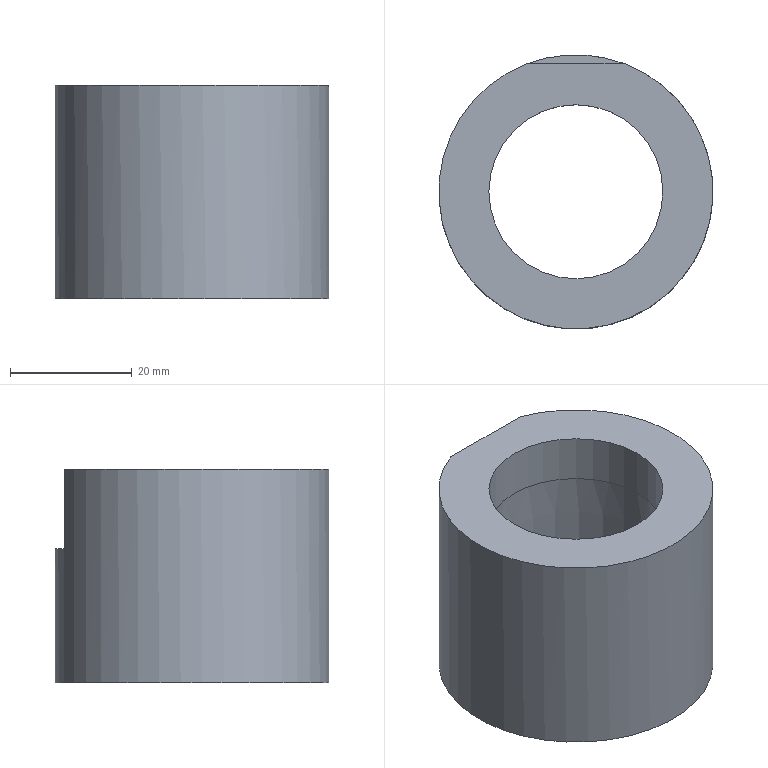Part | STEP file | lll_id4046_x_t | 1 solid | 7 faces | box 45 x 45 x 35 mm | volume 32145 mm3 | plane 4 | cylinder 2 | cone 1 | commonest cylinder face diameters 28.57 x1 45 x1
STEP:
#1=CARTESIAN_POINT('',(3205.477,-41.296,-35.));
#2=VERTEX_POINT('',#1);
#3=CARTESIAN_POINT('',(3205.477,-56.288,-35.));
#4=DIRECTION('',(0.,0.,-1.));
#5=DIRECTION('',(0.,1.,0.));
#6=AXIS2_PLACEMENT_3D('',#3,#4,#5);
#7=CIRCLE('',#6,14.992);
#8=EDGE_CURVE('',#2,#2,#7,.T.);
#9=ORIENTED_EDGE('',*,*,#8,.F.);
#10=EDGE_LOOP('',(#9));
#11=FACE_BOUND('',#10,.T.);
#12=CARTESIAN_POINT('',(3205.477,-33.788,-35.));
#13=VERTEX_POINT('',#12);
#14=CARTESIAN_POINT('',(3205.477,-56.288,-35.));
#15=DIRECTION('',(0.,0.,-1.));
#16=DIRECTION('',(0.,1.,0.));
#17=AXIS2_PLACEMENT_3D('',#14,#15,#16);
#18=CIRCLE('',#17,22.5);
#19=EDGE_CURVE('',#13,#13,#18,.T.);
#20=ORIENTED_EDGE('',*,*,#19,.T.);
#21=EDGE_LOOP('',(#20));
#22=FACE_BOUND('',#21,.T.);
#23=CARTESIAN_POINT('',(3199.977,-56.288,-35.));
#24=DIRECTION('',(0.,0.,-1.));
#25=DIRECTION('',(1.,0.,0.));
#26=AXIS2_PLACEMENT_3D('',#23,#24,#25);
#27=PLANE('',#26);
#28=ADVANCED_FACE('',(#11,#22),#27,.T.);
#29=CARTESIAN_POINT('',(3205.477,-42.003,-8.));
#30=VERTEX_POINT('',#29);
#31=CARTESIAN_POINT('',(3205.477,-56.288,-8.));
#32=DIRECTION('',(0.,0.,1.));
#33=DIRECTION('',(0.,1.,0.));
#34=AXIS2_PLACEMENT_3D('',#31,#32,#33);
#35=CIRCLE('',#34,14.285);
#36=EDGE_CURVE('',#30,#30,#35,.T.);
#37=ORIENTED_EDGE('',*,*,#36,.F.);
#38=EDGE_LOOP('',(#37));
#39=FACE_BOUND('',#38,.T.);
#40=CARTESIAN_POINT('',(3205.477,-42.003,0.00001711));
#41=VERTEX_POINT('',#40);
#42=CARTESIAN_POINT('',(3205.477,-56.288,0.00001711));
#43=DIRECTION('',(0.,0.,-1.));
#44=DIRECTION('',(0.,1.,0.));
#45=AXIS2_PLACEMENT_3D('',#42,#43,#44);
#46=CIRCLE('',#45,14.285);
#47=EDGE_CURVE('',#41,#41,#46,.T.);
#48=ORIENTED_EDGE('',*,*,#47,.F.);
#49=EDGE_LOOP('',(#48));
#50=FACE_BOUND('',#49,.T.);
#51=CARTESIAN_POINT('',(3205.477,-56.288,-2.4));
#52=DIRECTION('',(0.,0.,1.));
#53=DIRECTION('',(0.,1.,0.));
#54=AXIS2_PLACEMENT_3D('',#51,#52,#53);
#55=CYLINDRICAL_SURFACE('',#54,14.285);
#56=ADVANCED_FACE('',(#39,#50),#55,.F.);
#57=CARTESIAN_POINT('',(3213.554,-35.288,0.00001711));
#58=VERTEX_POINT('',#57);
#59=CARTESIAN_POINT('',(3197.399,-35.288,0.00001711));
#60=VERTEX_POINT('',#59);
#61=CARTESIAN_POINT('',(3205.477,-35.288,0.00001711));
#62=DIRECTION('',(-1.,0.,0.));
#63=VECTOR('',#62,1.);
#64=LINE('',#61,#63);
#65=EDGE_CURVE('',#58,#60,#64,.T.);
#66=ORIENTED_EDGE('',*,*,#65,.T.);
#67=CARTESIAN_POINT('',(3205.477,-56.288,0.00001711));
#68=DIRECTION('',(0.,0.,-1.));
#69=DIRECTION('',(0.,1.,0.));
#70=AXIS2_PLACEMENT_3D('',#67,#68,#69);
#71=CIRCLE('',#70,22.5);
#72=EDGE_CURVE('',#58,#60,#71,.T.);
#73=ORIENTED_EDGE('',*,*,#72,.F.);
#74=EDGE_LOOP('',(#66,#73));
#75=FACE_BOUND('',#74,.T.);
#76=ORIENTED_EDGE('',*,*,#47,.T.);
#77=EDGE_LOOP('',(#76));
#78=FACE_BOUND('',#77,.T.);
#79=CARTESIAN_POINT('',(3205.477,-56.288,0.00001711));
#80=DIRECTION('',(0.,0.,1.));
#81=DIRECTION('',(0.,-1.,0.));
#82=AXIS2_PLACEMENT_3D('',#79,#80,#81);
#83=PLANE('',#82);
#84=ADVANCED_FACE('',(#75,#78),#83,.T.);
#85=ORIENTED_EDGE('',*,*,#19,.F.);
#86=EDGE_LOOP('',(#85));
#87=FACE_BOUND('',#86,.T.);
#88=ORIENTED_EDGE('',*,*,#72,.T.);
#89=CARTESIAN_POINT('',(3197.399,-35.288,-13.));
#90=VERTEX_POINT('',#89);
#91=CARTESIAN_POINT('',(3197.399,-35.288,-15.));
#92=DIRECTION('',(0.,0.,-1.));
#93=VECTOR('',#92,1.);
#94=LINE('',#91,#93);
#95=EDGE_CURVE('',#60,#90,#94,.T.);
#96=ORIENTED_EDGE('',*,*,#95,.T.);
#97=CARTESIAN_POINT('',(3213.554,-35.288,-13.));
#98=VERTEX_POINT('',#97);
#99=CARTESIAN_POINT('',(3205.477,-56.288,-13.));
#100=DIRECTION('',(0.,0.,-1.));
#101=DIRECTION('',(0.,-1.,0.));
#102=AXIS2_PLACEMENT_3D('',#99,#100,#101);
#103=CIRCLE('',#102,22.5);
#104=EDGE_CURVE('',#90,#98,#103,.T.);
#105=ORIENTED_EDGE('',*,*,#104,.T.);
#106=CARTESIAN_POINT('',(3213.554,-35.288,-15.));
#107=DIRECTION('',(0.,0.,1.));
#108=VECTOR('',#107,1.);
#109=LINE('',#106,#108);
#110=EDGE_CURVE('',#98,#58,#109,.T.);
#111=ORIENTED_EDGE('',*,*,#110,.T.);
#112=EDGE_LOOP('',(#88,#96,#105,#111));
#113=FACE_BOUND('',#112,.T.);
#114=CARTESIAN_POINT('',(3205.477,-56.288,-15.));
#115=DIRECTION('',(0.,0.,-1.));
#116=DIRECTION('',(-1.,0.,0.));
#117=AXIS2_PLACEMENT_3D('',#114,#115,#116);
#118=CYLINDRICAL_SURFACE('',#117,22.5);
#119=ADVANCED_FACE('',(#87,#113),#118,.T.);
#120=CARTESIAN_POINT('',(3205.477,-35.288,-13.));
#121=DIRECTION('',(1.,0.,0.));
#122=VECTOR('',#121,1.);
#123=LINE('',#120,#122);
#124=EDGE_CURVE('',#90,#98,#123,.T.);
#125=ORIENTED_EDGE('',*,*,#124,.F.);
#126=ORIENTED_EDGE('',*,*,#95,.F.);
#127=ORIENTED_EDGE('',*,*,#65,.F.);
#128=ORIENTED_EDGE('',*,*,#110,.F.);
#129=EDGE_LOOP('',(#125,#126,#127,#128));
#130=FACE_OUTER_BOUND('',#129,.T.);
#131=CARTESIAN_POINT('',(3187.084,-35.288,-17.5));
#132=DIRECTION('',(0.,-1.,0.));
#133=DIRECTION('',(0.,0.,-1.));
#134=AXIS2_PLACEMENT_3D('',#131,#132,#133);
#135=PLANE('',#134);
#136=ADVANCED_FACE('',(#130),#135,.F.);
#137=ORIENTED_EDGE('',*,*,#104,.F.);
#138=ORIENTED_EDGE('',*,*,#124,.T.);
#139=EDGE_LOOP('',(#137,#138));
#140=FACE_OUTER_BOUND('',#139,.T.);
#141=CARTESIAN_POINT('',(3205.477,-56.288,-13.));
#142=DIRECTION('',(0.,0.,1.));
#143=DIRECTION('',(0.,-1.,0.));
#144=AXIS2_PLACEMENT_3D('',#141,#142,#143);
#145=PLANE('',#144);
#146=ADVANCED_FACE('',(#140),#145,.T.);
#147=ORIENTED_EDGE('',*,*,#8,.T.);
#148=EDGE_LOOP('',(#147));
#149=FACE_BOUND('',#148,.T.);
#150=ORIENTED_EDGE('',*,*,#36,.T.);
#151=EDGE_LOOP('',(#150));
#152=FACE_BOUND('',#151,.T.);
#153=CARTESIAN_POINT('',(3205.477,-56.288,-8.));
#154=DIRECTION('',(0.,0.,-1.));
#155=DIRECTION('',(0.,1.,0.));
#156=AXIS2_PLACEMENT_3D('',#153,#154,#155);
#157=CONICAL_SURFACE('',#156,14.285,1.5);
#158=ADVANCED_FACE('',(#149,#152),#157,.F.);
#159=CLOSED_SHELL('',(#28,#56,#84,#119,#136,#146,#158));
#160=MANIFOLD_SOLID_BREP('',#159);
#161=(LENGTH_UNIT()NAMED_UNIT(*)SI_UNIT(.MILLI.,.METRE.));
#162=UNCERTAINTY_MEASURE_WITH_UNIT(LENGTH_MEASURE(0.00002),#161,'','');
#163=(NAMED_UNIT(*)PLANE_ANGLE_UNIT()SI_UNIT($,.RADIAN.));
#164=PLANE_ANGLE_MEASURE_WITH_UNIT(PLANE_ANGLE_MEASURE(0.01745),#163);
#165=DIMENSIONAL_EXPONENTS(0.,0.,0.,0.,0.,0.,0.);
#166=(CONVERSION_BASED_UNIT('DEGREE',#164)NAMED_UNIT(#165)PLANE_ANGLE_UNIT());
#167=(NAMED_UNIT(*)SI_UNIT($,.STERADIAN.)SOLID_ANGLE_UNIT());
#168=(GEOMETRIC_REPRESENTATION_CONTEXT(3)GLOBAL_UNCERTAINTY_ASSIGNED_CONTEXT((#162))GLOBAL_UNIT_ASSIGNED_CONTEXT((#161,#166,#167))REPRESENTATION_CONTEXT('',''));
#169=ADVANCED_BREP_SHAPE_REPRESENTATION('',(#160),#168);